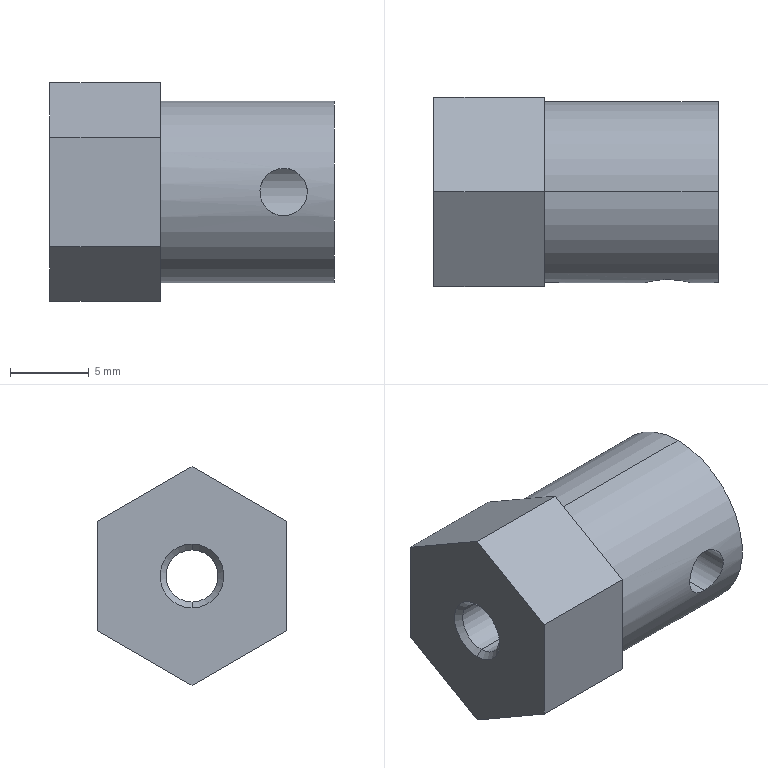Part | SolidWorks | features ICE 3, Extrusion 1, HoleWzd 1 | 1 solid | 20 faces | box 18 x 12 x 13.856 mm | volume 1793 mm3 | plane 10 | cylinder 8 | cone 2 | commonest cylinder face diameters 3 x2 3.3 x2 4 x2 11.5 x2
STEP:
#1=CARTESIAN_POINT('',(14.8,-5.551,-1.5));
#2=VERTEX_POINT('',#1);
#3=CARTESIAN_POINT('',(14.8,-5.551,1.5));
#4=VERTEX_POINT('',#3);
#5=CARTESIAN_POINT('',(14.8,-5.551,-1.5));
#6=CARTESIAN_POINT('',(14.604,-5.551,-1.5));
#7=CARTESIAN_POINT('',(14.406,-5.562,-1.46));
#8=CARTESIAN_POINT('',(14.135,-5.59,-1.348));
#9=CARTESIAN_POINT('',(14.047,-5.601,-1.301));
#10=CARTESIAN_POINT('',(13.884,-5.625,-1.192));
#11=CARTESIAN_POINT('',(13.809,-5.638,-1.13));
#12=CARTESIAN_POINT('',(13.671,-5.664,-0.992));
#13=CARTESIAN_POINT('',(13.608,-5.677,-0.9153));
#14=CARTESIAN_POINT('',(13.499,-5.701,-0.7534));
#15=CARTESIAN_POINT('',(13.453,-5.712,-0.6674));
#16=CARTESIAN_POINT('',(13.339,-5.739,-0.3935));
#17=CARTESIAN_POINT('',(13.3,-5.75,-0.1982));
#18=CARTESIAN_POINT('',(13.3,-5.75,0.09853));
#19=CARTESIAN_POINT('',(13.31,-5.747,0.1962));
#20=CARTESIAN_POINT('',(13.348,-5.738,0.389));
#21=CARTESIAN_POINT('',(13.377,-5.73,0.4847));
#22=CARTESIAN_POINT('',(13.49,-5.703,0.756));
#23=CARTESIAN_POINT('',(13.601,-5.677,0.9225));
#24=CARTESIAN_POINT('',(13.876,-5.626,1.198));
#25=CARTESIAN_POINT('',(14.043,-5.599,1.31));
#26=CARTESIAN_POINT('',(14.314,-5.571,1.422));
#27=CARTESIAN_POINT('',(14.409,-5.564,1.452));
#28=CARTESIAN_POINT('',(14.602,-5.554,1.49));
#29=CARTESIAN_POINT('',(14.7,-5.551,1.5));
#30=CARTESIAN_POINT('',(14.8,-5.551,1.5));
#31=B_SPLINE_CURVE_WITH_KNOTS('',3,(#5,#6,#7,#8,#9,#10,#11,#12,#13,#14,#15,#16,#17,#18,#19,#20,#21,#22,#23,#24,#25,#26,#27,#28,#29,#30),.UNSPECIFIED.,.F.,.F.,(4,2,2,2,2,2,2,2,2,2,2,2,4),(0.00471,0.005299,0.005593,0.005887,0.006182,0.006476,0.007064,0.007359,0.007653,0.008242,0.00883,0.009125,0.009419),.UNSPECIFIED.);
#32=EDGE_CURVE('',#2,#4,#31,.T.);
#33=ORIENTED_EDGE('',*,*,#32,.F.);
#34=CARTESIAN_POINT('',(14.8,-1.323,-1.5));
#35=VERTEX_POINT('',#34);
#36=CARTESIAN_POINT('',(14.8,-6.,-1.5));
#37=DIRECTION('',(0.,1.,0.));
#38=VECTOR('',#37,1000.);
#39=LINE('',#36,#38);
#40=EDGE_CURVE('',#2,#35,#39,.T.);
#41=ORIENTED_EDGE('',*,*,#40,.T.);
#42=CARTESIAN_POINT('',(14.8,-1.323,1.5));
#43=VERTEX_POINT('',#42);
#44=CARTESIAN_POINT('',(14.8,-1.323,1.5));
#45=CARTESIAN_POINT('',(14.696,-1.323,1.5));
#46=CARTESIAN_POINT('',(14.595,-1.335,1.489));
#47=CARTESIAN_POINT('',(14.399,-1.379,1.449));
#48=CARTESIAN_POINT('',(14.303,-1.411,1.419));
#49=CARTESIAN_POINT('',(14.037,-1.518,1.306));
#50=CARTESIAN_POINT('',(13.88,-1.608,1.2));
#51=CARTESIAN_POINT('',(13.679,-1.733,1.002));
#52=CARTESIAN_POINT('',(13.618,-1.774,0.9281));
#53=CARTESIAN_POINT('',(13.51,-1.847,0.7712));
#54=CARTESIAN_POINT('',(13.463,-1.881,0.6872));
#55=CARTESIAN_POINT('',(13.345,-1.966,0.4152));
#56=CARTESIAN_POINT('',(13.3,-2.,0.209));
#57=CARTESIAN_POINT('',(13.3,-2.,-0.2028));
#58=CARTESIAN_POINT('',(13.343,-1.967,-0.4078));
#59=CARTESIAN_POINT('',(13.499,-1.855,-0.7725));
#60=CARTESIAN_POINT('',(13.61,-1.776,-0.9331));
#61=CARTESIAN_POINT('',(13.812,-1.65,-1.133));
#62=CARTESIAN_POINT('',(13.884,-1.608,-1.192));
#63=CARTESIAN_POINT('',(14.04,-1.524,-1.297));
#64=CARTESIAN_POINT('',(14.124,-1.483,-1.343));
#65=CARTESIAN_POINT('',(14.391,-1.375,-1.456));
#66=CARTESIAN_POINT('',(14.592,-1.323,-1.5));
#67=CARTESIAN_POINT('',(14.8,-1.323,-1.5));
#68=B_SPLINE_CURVE_WITH_KNOTS('',3,(#44,#45,#46,#47,#48,#49,#50,#51,#52,#53,#54,#55,#56,#57,#58,#59,#60,#61,#62,#63,#64,#65,#66,#67),.UNSPECIFIED.,.F.,.F.,(4,2,2,2,2,2,2,2,2,2,2,4),(0.,0.0003062,0.0006124,0.001225,0.001531,0.001837,0.00245,0.003062,0.003675,0.003981,0.004287,0.004899),.UNSPECIFIED.);
#69=EDGE_CURVE('',#43,#35,#68,.T.);
#70=ORIENTED_EDGE('',*,*,#69,.F.);
#71=CARTESIAN_POINT('',(14.8,-6.,1.5));
#72=DIRECTION('',(0.,1.,0.));
#73=VECTOR('',#72,1000.);
#74=LINE('',#71,#73);
#75=EDGE_CURVE('',#4,#43,#74,.T.);
#76=ORIENTED_EDGE('',*,*,#75,.F.);
#77=EDGE_LOOP('',(#33,#41,#70,#76));
#78=FACE_OUTER_BOUND('',#77,.T.);
#79=CARTESIAN_POINT('',(14.8,-6.,0.));
#80=DIRECTION('',(0.,1.,0.));
#81=DIRECTION('',(0.,0.,1.));
#82=AXIS2_PLACEMENT_3D('',#79,#80,#81);
#83=CYLINDRICAL_SURFACE('',#82,1.5);
#84=ADVANCED_FACE('',(#78),#83,.F.);
#85=CARTESIAN_POINT('',(0.375,0.,-1.65));
#86=VERTEX_POINT('',#85);
#87=CARTESIAN_POINT('',(0.375,0.,1.65));
#88=VERTEX_POINT('',#87);
#89=CARTESIAN_POINT('',(0.375,0.,0.));
#90=DIRECTION('',(-1.,0.,0.));
#91=DIRECTION('',(0.,0.,1.));
#92=AXIS2_PLACEMENT_3D('',#89,#90,#91);
#93=CIRCLE('',#92,1.65);
#94=EDGE_CURVE('',#86,#88,#93,.T.);
#95=ORIENTED_EDGE('',*,*,#94,.F.);
#96=CARTESIAN_POINT('',(0.,0.,-2.025));
#97=VERTEX_POINT('',#96);
#98=CARTESIAN_POINT('',(0.,0.,-2.025));
#99=DIRECTION('',(-0.7071,0.,-0.7071));
#100=VECTOR('',#99,1000.);
#101=LINE('',#98,#100);
#102=EDGE_CURVE('',#86,#97,#101,.T.);
#103=ORIENTED_EDGE('',*,*,#102,.T.);
#104=CARTESIAN_POINT('',(0.,0.,2.025));
#105=VERTEX_POINT('',#104);
#106=CARTESIAN_POINT('',(0.,0.,0.));
#107=DIRECTION('',(-1.,0.,0.));
#108=DIRECTION('',(0.,0.,1.));
#109=AXIS2_PLACEMENT_3D('',#106,#107,#108);
#110=CIRCLE('',#109,2.025);
#111=EDGE_CURVE('',#97,#105,#110,.T.);
#112=ORIENTED_EDGE('',*,*,#111,.T.);
#113=CARTESIAN_POINT('',(0.,0.,2.025));
#114=DIRECTION('',(-0.7071,0.,0.7071));
#115=VECTOR('',#114,1000.);
#116=LINE('',#113,#115);
#117=EDGE_CURVE('',#88,#105,#116,.T.);
#118=ORIENTED_EDGE('',*,*,#117,.F.);
#119=EDGE_LOOP('',(#95,#103,#112,#118));
#120=FACE_OUTER_BOUND('',#119,.T.);
#121=CARTESIAN_POINT('',(0.,0.,0.));
#122=DIRECTION('',(-1.,0.,0.));
#123=DIRECTION('',(0.,0.,1.));
#124=AXIS2_PLACEMENT_3D('',#121,#122,#123);
#125=CONICAL_SURFACE('',#124,2.025,0.7854);
#126=ADVANCED_FACE('',(#120),#125,.F.);
#127=CARTESIAN_POINT('',(8.,0.,1.65));
#128=VERTEX_POINT('',#127);
#129=CARTESIAN_POINT('',(8.,0.,-1.65));
#130=VERTEX_POINT('',#129);
#131=CARTESIAN_POINT('',(8.,0.,0.));
#132=DIRECTION('',(1.,0.,0.));
#133=DIRECTION('',(0.,0.,-1.));
#134=AXIS2_PLACEMENT_3D('',#131,#132,#133);
#135=CIRCLE('',#134,1.65);
#136=EDGE_CURVE('',#128,#130,#135,.T.);
#137=ORIENTED_EDGE('',*,*,#136,.T.);
#138=CARTESIAN_POINT('',(0.,0.,-1.65));
#139=DIRECTION('',(-1.,0.,0.));
#140=VECTOR('',#139,1000.);
#141=LINE('',#138,#140);
#142=EDGE_CURVE('',#130,#86,#141,.T.);
#143=ORIENTED_EDGE('',*,*,#142,.T.);
#144=ORIENTED_EDGE('',*,*,#94,.T.);
#145=CARTESIAN_POINT('',(0.,0.,1.65));
#146=DIRECTION('',(-1.,0.,0.));
#147=VECTOR('',#146,1000.);
#148=LINE('',#145,#147);
#149=EDGE_CURVE('',#128,#88,#148,.T.);
#150=ORIENTED_EDGE('',*,*,#149,.F.);
#151=EDGE_LOOP('',(#137,#143,#144,#150));
#152=FACE_OUTER_BOUND('',#151,.T.);
#153=CARTESIAN_POINT('',(0.,0.,0.));
#154=DIRECTION('',(-1.,0.,0.));
#155=DIRECTION('',(0.,0.,1.));
#156=AXIS2_PLACEMENT_3D('',#153,#154,#155);
#157=CYLINDRICAL_SURFACE('',#156,1.65);
#158=ADVANCED_FACE('',(#152),#157,.F.);
#159=ORIENTED_EDGE('',*,*,#69,.T.);
#160=CARTESIAN_POINT('',(14.8,-1.323,-1.5));
#161=CARTESIAN_POINT('',(15.007,-1.323,-1.5));
#162=CARTESIAN_POINT('',(15.21,-1.375,-1.456));
#163=CARTESIAN_POINT('',(15.563,-1.519,-1.306));
#164=CARTESIAN_POINT('',(15.72,-1.608,-1.199));
#165=CARTESIAN_POINT('',(15.921,-1.733,-1.001));
#166=CARTESIAN_POINT('',(15.983,-1.774,-0.9276));
#167=CARTESIAN_POINT('',(16.09,-1.848,-0.7707));
#168=CARTESIAN_POINT('',(16.137,-1.881,-0.6867));
#169=CARTESIAN_POINT('',(16.255,-1.966,-0.4153));
#170=CARTESIAN_POINT('',(16.3,-2.,-0.2091));
#171=CARTESIAN_POINT('',(16.3,-2.,0.2031));
#172=CARTESIAN_POINT('',(16.257,-1.967,0.4079));
#173=CARTESIAN_POINT('',(16.101,-1.855,0.7722));
#174=CARTESIAN_POINT('',(15.99,-1.776,0.9327));
#175=CARTESIAN_POINT('',(15.788,-1.65,1.132));
#176=CARTESIAN_POINT('',(15.716,-1.608,1.192));
#177=CARTESIAN_POINT('',(15.56,-1.524,1.296));
#178=CARTESIAN_POINT('',(15.476,-1.483,1.342));
#179=CARTESIAN_POINT('',(15.21,-1.375,1.456));
#180=CARTESIAN_POINT('',(15.008,-1.323,1.5));
#181=CARTESIAN_POINT('',(14.8,-1.323,1.5));
#182=B_SPLINE_CURVE_WITH_KNOTS('',3,(#160,#161,#162,#163,#164,#165,#166,#167,#168,#169,#170,#171,#172,#173,#174,#175,#176,#177,#178,#179,#180,#181),.UNSPECIFIED.,.F.,.F.,(4,2,2,2,2,2,2,2,2,2,4),(0.004899,0.005511,0.006122,0.006427,0.006733,0.007344,0.007956,0.008567,0.008872,0.009178,0.009789),.UNSPECIFIED.);
#183=EDGE_CURVE('',#35,#43,#182,.T.);
#184=ORIENTED_EDGE('',*,*,#183,.T.);
#185=EDGE_LOOP('',(#159,#184));
#186=FACE_BOUND('',#185,.T.);
#187=CARTESIAN_POINT('',(8.,0.,2.));
#188=VERTEX_POINT('',#187);
#189=CARTESIAN_POINT('',(8.,0.,-2.));
#190=VERTEX_POINT('',#189);
#191=CARTESIAN_POINT('',(8.,0.,0.));
#192=DIRECTION('',(1.,0.,0.));
#193=DIRECTION('',(0.,0.,-1.));
#194=AXIS2_PLACEMENT_3D('',#191,#192,#193);
#195=CIRCLE('',#194,2.);
#196=EDGE_CURVE('',#188,#190,#195,.T.);
#197=ORIENTED_EDGE('',*,*,#196,.F.);
#198=CARTESIAN_POINT('',(18.,0.,2.));
#199=VERTEX_POINT('',#198);
#200=CARTESIAN_POINT('',(8.,0.,2.));
#201=DIRECTION('',(1.,0.,0.));
#202=VECTOR('',#201,1000.);
#203=LINE('',#200,#202);
#204=EDGE_CURVE('',#188,#199,#203,.T.);
#205=ORIENTED_EDGE('',*,*,#204,.T.);
#206=CARTESIAN_POINT('',(18.,0.,-2.));
#207=VERTEX_POINT('',#206);
#208=CARTESIAN_POINT('',(18.,0.,0.));
#209=DIRECTION('',(1.,0.,0.));
#210=DIRECTION('',(0.,0.,-1.));
#211=AXIS2_PLACEMENT_3D('',#208,#209,#210);
#212=CIRCLE('',#211,2.);
#213=EDGE_CURVE('',#199,#207,#212,.T.);
#214=ORIENTED_EDGE('',*,*,#213,.T.);
#215=CARTESIAN_POINT('',(8.,0.,-2.));
#216=DIRECTION('',(1.,0.,0.));
#217=VECTOR('',#216,1000.);
#218=LINE('',#215,#217);
#219=EDGE_CURVE('',#190,#207,#218,.T.);
#220=ORIENTED_EDGE('',*,*,#219,.F.);
#221=EDGE_LOOP('',(#197,#205,#214,#220));
#222=FACE_OUTER_BOUND('',#221,.T.);
#223=CARTESIAN_POINT('',(8.,0.,0.));
#224=DIRECTION('',(1.,0.,0.));
#225=DIRECTION('',(0.,0.,-1.));
#226=AXIS2_PLACEMENT_3D('',#223,#224,#225);
#227=CYLINDRICAL_SURFACE('',#226,2.);
#228=ADVANCED_FACE('',(#186,#222),#227,.F.);
#229=CARTESIAN_POINT('',(18.,0.,-5.75));
#230=VERTEX_POINT('',#229);
#231=CARTESIAN_POINT('',(18.,0.,5.75));
#232=VERTEX_POINT('',#231);
#233=CARTESIAN_POINT('',(18.,0.,0.));
#234=DIRECTION('',(1.,0.,0.));
#235=DIRECTION('',(0.,0.,-1.));
#236=AXIS2_PLACEMENT_3D('',#233,#234,#235);
#237=CIRCLE('',#236,5.75);
#238=EDGE_CURVE('',#230,#232,#237,.T.);
#239=ORIENTED_EDGE('',*,*,#238,.F.);
#240=CARTESIAN_POINT('',(7.,0.,-5.75));
#241=VERTEX_POINT('',#240);
#242=CARTESIAN_POINT('',(18.,0.,-5.75));
#243=DIRECTION('',(-1.,0.,0.));
#244=VECTOR('',#243,1000.);
#245=LINE('',#242,#244);
#246=EDGE_CURVE('',#230,#241,#245,.T.);
#247=ORIENTED_EDGE('',*,*,#246,.T.);
#248=CARTESIAN_POINT('',(7.,0.,5.75));
#249=VERTEX_POINT('',#248);
#250=CARTESIAN_POINT('',(7.,0.,0.));
#251=DIRECTION('',(1.,0.,0.));
#252=DIRECTION('',(0.,0.,-1.));
#253=AXIS2_PLACEMENT_3D('',#250,#251,#252);
#254=CIRCLE('',#253,5.75);
#255=EDGE_CURVE('',#241,#249,#254,.T.);
#256=ORIENTED_EDGE('',*,*,#255,.T.);
#257=CARTESIAN_POINT('',(18.,0.,5.75));
#258=DIRECTION('',(-1.,0.,0.));
#259=VECTOR('',#258,1000.);
#260=LINE('',#257,#259);
#261=EDGE_CURVE('',#232,#249,#260,.T.);
#262=ORIENTED_EDGE('',*,*,#261,.F.);
#263=EDGE_LOOP('',(#239,#247,#256,#262));
#264=FACE_OUTER_BOUND('',#263,.T.);
#265=CARTESIAN_POINT('',(18.,0.,0.));
#266=DIRECTION('',(-1.,0.,0.));
#267=DIRECTION('',(0.,0.,1.));
#268=AXIS2_PLACEMENT_3D('',#265,#266,#267);
#269=CYLINDRICAL_SURFACE('',#268,5.75);
#270=ADVANCED_FACE('',(#264),#269,.T.);
#271=CARTESIAN_POINT('',(0.,-6.,-3.464));
#272=VERTEX_POINT('',#271);
#273=CARTESIAN_POINT('',(0.,0.,-6.928));
#274=VERTEX_POINT('',#273);
#275=CARTESIAN_POINT('',(0.,-6.,-3.464));
#276=DIRECTION('',(0.,0.866,-0.5));
#277=VECTOR('',#276,1000.);
#278=LINE('',#275,#277);
#279=EDGE_CURVE('',#272,#274,#278,.T.);
#280=ORIENTED_EDGE('',*,*,#279,.F.);
#281=CARTESIAN_POINT('',(0.,-6.,3.464));
#282=VERTEX_POINT('',#281);
#283=CARTESIAN_POINT('',(0.,-6.,3.464));
#284=DIRECTION('',(0.,0.,-1.));
#285=VECTOR('',#284,1000.);
#286=LINE('',#283,#285);
#287=EDGE_CURVE('',#282,#272,#286,.T.);
#288=ORIENTED_EDGE('',*,*,#287,.F.);
#289=CARTESIAN_POINT('',(0.,0.,6.928));
#290=VERTEX_POINT('',#289);
#291=CARTESIAN_POINT('',(0.,0.,6.928));
#292=DIRECTION('',(0.,-0.866,-0.5));
#293=VECTOR('',#292,1000.);
#294=LINE('',#291,#293);
#295=EDGE_CURVE('',#290,#282,#294,.T.);
#296=ORIENTED_EDGE('',*,*,#295,.F.);
#297=CARTESIAN_POINT('',(0.,6.,3.464));
#298=VERTEX_POINT('',#297);
#299=CARTESIAN_POINT('',(0.,6.,3.464));
#300=DIRECTION('',(0.,-0.866,0.5));
#301=VECTOR('',#300,1000.);
#302=LINE('',#299,#301);
#303=EDGE_CURVE('',#298,#290,#302,.T.);
#304=ORIENTED_EDGE('',*,*,#303,.F.);
#305=CARTESIAN_POINT('',(0.,6.,-3.464));
#306=VERTEX_POINT('',#305);
#307=CARTESIAN_POINT('',(0.,6.,-3.464));
#308=DIRECTION('',(0.,0.,1.));
#309=VECTOR('',#308,1000.);
#310=LINE('',#307,#309);
#311=EDGE_CURVE('',#306,#298,#310,.T.);
#312=ORIENTED_EDGE('',*,*,#311,.F.);
#313=CARTESIAN_POINT('',(0.,0.,-6.928));
#314=DIRECTION('',(0.,0.866,0.5));
#315=VECTOR('',#314,1000.);
#316=LINE('',#313,#315);
#317=EDGE_CURVE('',#274,#306,#316,.T.);
#318=ORIENTED_EDGE('',*,*,#317,.F.);
#319=EDGE_LOOP('',(#280,#288,#296,#304,#312,#318));
#320=FACE_OUTER_BOUND('',#319,.T.);
#321=CARTESIAN_POINT('',(0.,0.,0.));
#322=DIRECTION('',(-1.,0.,0.));
#323=DIRECTION('',(0.,0.,1.));
#324=AXIS2_PLACEMENT_3D('',#321,#322,#323);
#325=CIRCLE('',#324,2.025);
#326=EDGE_CURVE('',#105,#97,#325,.T.);
#327=ORIENTED_EDGE('',*,*,#326,.F.);
#328=ORIENTED_EDGE('',*,*,#111,.F.);
#329=EDGE_LOOP('',(#327,#328));
#330=FACE_BOUND('',#329,.T.);
#331=CARTESIAN_POINT('',(0.,0.,0.));
#332=DIRECTION('',(1.,0.,0.));
#333=DIRECTION('',(0.,0.,-1.));
#334=AXIS2_PLACEMENT_3D('',#331,#332,#333);
#335=PLANE('',#334);
#336=ADVANCED_FACE('',(#320,#330),#335,.F.);
#337=ORIENTED_EDGE('',*,*,#279,.T.);
#338=CARTESIAN_POINT('',(7.,0.,-6.928));
#339=VERTEX_POINT('',#338);
#340=CARTESIAN_POINT('',(7.,0.,-6.928));
#341=DIRECTION('',(-1.,0.,0.));
#342=VECTOR('',#341,1000.);
#343=LINE('',#340,#342);
#344=EDGE_CURVE('',#339,#274,#343,.T.);
#345=ORIENTED_EDGE('',*,*,#344,.F.);
#346=CARTESIAN_POINT('',(7.,-6.,-3.464));
#347=VERTEX_POINT('',#346);
#348=CARTESIAN_POINT('',(7.,-6.,-3.464));
#349=DIRECTION('',(0.,0.866,-0.5));
#350=VECTOR('',#349,1000.);
#351=LINE('',#348,#350);
#352=EDGE_CURVE('',#347,#339,#351,.T.);
#353=ORIENTED_EDGE('',*,*,#352,.F.);
#354=CARTESIAN_POINT('',(7.,-6.,-3.464));
#355=DIRECTION('',(-1.,0.,0.));
#356=VECTOR('',#355,1000.);
#357=LINE('',#354,#356);
#358=EDGE_CURVE('',#347,#272,#357,.T.);
#359=ORIENTED_EDGE('',*,*,#358,.T.);
#360=EDGE_LOOP('',(#337,#345,#353,#359));
#361=FACE_OUTER_BOUND('',#360,.T.);
#362=CARTESIAN_POINT('',(7.,-6.,-3.464));
#363=DIRECTION('',(0.,0.5,0.866));
#364=DIRECTION('',(0.,-0.866,0.5));
#365=AXIS2_PLACEMENT_3D('',#362,#363,#364);
#366=PLANE('',#365);
#367=ADVANCED_FACE('',(#361),#366,.F.);
#368=ORIENTED_EDGE('',*,*,#317,.T.);
#369=CARTESIAN_POINT('',(7.,6.,-3.464));
#370=VERTEX_POINT('',#369);
#371=CARTESIAN_POINT('',(7.,6.,-3.464));
#372=DIRECTION('',(-1.,0.,0.));
#373=VECTOR('',#372,1000.);
#374=LINE('',#371,#373);
#375=EDGE_CURVE('',#370,#306,#374,.T.);
#376=ORIENTED_EDGE('',*,*,#375,.F.);
#377=CARTESIAN_POINT('',(7.,0.,-6.928));
#378=DIRECTION('',(0.,0.866,0.5));
#379=VECTOR('',#378,1000.);
#380=LINE('',#377,#379);
#381=EDGE_CURVE('',#339,#370,#380,.T.);
#382=ORIENTED_EDGE('',*,*,#381,.F.);
#383=ORIENTED_EDGE('',*,*,#344,.T.);
#384=EDGE_LOOP('',(#368,#376,#382,#383));
#385=FACE_OUTER_BOUND('',#384,.T.);
#386=CARTESIAN_POINT('',(7.,0.,-6.928));
#387=DIRECTION('',(0.,-0.5,0.866));
#388=DIRECTION('',(0.,-0.866,-0.5));
#389=AXIS2_PLACEMENT_3D('',#386,#387,#388);
#390=PLANE('',#389);
#391=ADVANCED_FACE('',(#385),#390,.F.);
#392=ORIENTED_EDGE('',*,*,#311,.T.);
#393=CARTESIAN_POINT('',(7.,6.,3.464));
#394=VERTEX_POINT('',#393);
#395=CARTESIAN_POINT('',(7.,6.,3.464));
#396=DIRECTION('',(-1.,0.,0.));
#397=VECTOR('',#396,1000.);
#398=LINE('',#395,#397);
#399=EDGE_CURVE('',#394,#298,#398,.T.);
#400=ORIENTED_EDGE('',*,*,#399,.F.);
#401=CARTESIAN_POINT('',(7.,6.,-3.464));
#402=DIRECTION('',(0.,0.,1.));
#403=VECTOR('',#402,1000.);
#404=LINE('',#401,#403);
#405=EDGE_CURVE('',#370,#394,#404,.T.);
#406=ORIENTED_EDGE('',*,*,#405,.F.);
#407=ORIENTED_EDGE('',*,*,#375,.T.);
#408=EDGE_LOOP('',(#392,#400,#406,#407));
#409=FACE_OUTER_BOUND('',#408,.T.);
#410=CARTESIAN_POINT('',(7.,6.,-3.464));
#411=DIRECTION('',(0.,-1.,0.));
#412=DIRECTION('',(0.,0.,-1.));
#413=AXIS2_PLACEMENT_3D('',#410,#411,#412);
#414=PLANE('',#413);
#415=ADVANCED_FACE('',(#409),#414,.F.);
#416=ORIENTED_EDGE('',*,*,#303,.T.);
#417=CARTESIAN_POINT('',(7.,0.,6.928));
#418=VERTEX_POINT('',#417);
#419=CARTESIAN_POINT('',(7.,0.,6.928));
#420=DIRECTION('',(-1.,0.,0.));
#421=VECTOR('',#420,1000.);
#422=LINE('',#419,#421);
#423=EDGE_CURVE('',#418,#290,#422,.T.);
#424=ORIENTED_EDGE('',*,*,#423,.F.);
#425=CARTESIAN_POINT('',(7.,6.,3.464));
#426=DIRECTION('',(0.,-0.866,0.5));
#427=VECTOR('',#426,1000.);
#428=LINE('',#425,#427);
#429=EDGE_CURVE('',#394,#418,#428,.T.);
#430=ORIENTED_EDGE('',*,*,#429,.F.);
#431=ORIENTED_EDGE('',*,*,#399,.T.);
#432=EDGE_LOOP('',(#416,#424,#430,#431));
#433=FACE_OUTER_BOUND('',#432,.T.);
#434=CARTESIAN_POINT('',(7.,6.,3.464));
#435=DIRECTION('',(0.,-0.5,-0.866));
#436=DIRECTION('',(0.,0.866,-0.5));
#437=AXIS2_PLACEMENT_3D('',#434,#435,#436);
#438=PLANE('',#437);
#439=ADVANCED_FACE('',(#433),#438,.F.);
#440=ORIENTED_EDGE('',*,*,#295,.T.);
#441=CARTESIAN_POINT('',(7.,-6.,3.464));
#442=VERTEX_POINT('',#441);
#443=CARTESIAN_POINT('',(7.,-6.,3.464));
#444=DIRECTION('',(-1.,0.,0.));
#445=VECTOR('',#444,1000.);
#446=LINE('',#443,#445);
#447=EDGE_CURVE('',#442,#282,#446,.T.);
#448=ORIENTED_EDGE('',*,*,#447,.F.);
#449=CARTESIAN_POINT('',(7.,0.,6.928));
#450=DIRECTION('',(0.,-0.866,-0.5));
#451=VECTOR('',#450,1000.);
#452=LINE('',#449,#451);
#453=EDGE_CURVE('',#418,#442,#452,.T.);
#454=ORIENTED_EDGE('',*,*,#453,.F.);
#455=ORIENTED_EDGE('',*,*,#423,.T.);
#456=EDGE_LOOP('',(#440,#448,#454,#455));
#457=FACE_OUTER_BOUND('',#456,.T.);
#458=CARTESIAN_POINT('',(7.,0.,6.928));
#459=DIRECTION('',(0.,0.5,-0.866));
#460=DIRECTION('',(0.,0.866,0.5));
#461=AXIS2_PLACEMENT_3D('',#458,#459,#460);
#462=PLANE('',#461);
#463=ADVANCED_FACE('',(#457),#462,.F.);
#464=ORIENTED_EDGE('',*,*,#287,.T.);
#465=ORIENTED_EDGE('',*,*,#358,.F.);
#466=CARTESIAN_POINT('',(7.,-6.,3.464));
#467=DIRECTION('',(0.,0.,-1.));
#468=VECTOR('',#467,1000.);
#469=LINE('',#466,#468);
#470=EDGE_CURVE('',#442,#347,#469,.T.);
#471=ORIENTED_EDGE('',*,*,#470,.F.);
#472=ORIENTED_EDGE('',*,*,#447,.T.);
#473=EDGE_LOOP('',(#464,#465,#471,#472));
#474=FACE_OUTER_BOUND('',#473,.T.);
#475=CARTESIAN_POINT('',(7.,-6.,3.464));
#476=DIRECTION('',(0.,1.,0.));
#477=DIRECTION('',(0.,0.,1.));
#478=AXIS2_PLACEMENT_3D('',#475,#476,#477);
#479=PLANE('',#478);
#480=ADVANCED_FACE('',(#474),#479,.F.);
#481=CARTESIAN_POINT('',(7.,0.,0.));
#482=DIRECTION('',(1.,0.,0.));
#483=DIRECTION('',(0.,0.,-1.));
#484=AXIS2_PLACEMENT_3D('',#481,#482,#483);
#485=CIRCLE('',#484,5.75);
#486=EDGE_CURVE('',#249,#241,#485,.T.);
#487=ORIENTED_EDGE('',*,*,#486,.F.);
#488=ORIENTED_EDGE('',*,*,#255,.F.);
#489=EDGE_LOOP('',(#487,#488));
#490=FACE_BOUND('',#489,.T.);
#491=ORIENTED_EDGE('',*,*,#352,.T.);
#492=ORIENTED_EDGE('',*,*,#381,.T.);
#493=ORIENTED_EDGE('',*,*,#405,.T.);
#494=ORIENTED_EDGE('',*,*,#429,.T.);
#495=ORIENTED_EDGE('',*,*,#453,.T.);
#496=ORIENTED_EDGE('',*,*,#470,.T.);
#497=EDGE_LOOP('',(#491,#492,#493,#494,#495,#496));
#498=FACE_OUTER_BOUND('',#497,.T.);
#499=CARTESIAN_POINT('',(7.,0.,0.));
#500=DIRECTION('',(1.,0.,0.));
#501=DIRECTION('',(0.,0.,-1.));
#502=AXIS2_PLACEMENT_3D('',#499,#500,#501);
#503=PLANE('',#502);
#504=ADVANCED_FACE('',(#490,#498),#503,.T.);
#505=ORIENTED_EDGE('',*,*,#246,.F.);
#506=CARTESIAN_POINT('',(18.,0.,0.));
#507=DIRECTION('',(1.,0.,0.));
#508=DIRECTION('',(0.,0.,-1.));
#509=AXIS2_PLACEMENT_3D('',#506,#507,#508);
#510=CIRCLE('',#509,5.75);
#511=EDGE_CURVE('',#232,#230,#510,.T.);
#512=ORIENTED_EDGE('',*,*,#511,.F.);
#513=ORIENTED_EDGE('',*,*,#261,.T.);
#514=ORIENTED_EDGE('',*,*,#486,.T.);
#515=EDGE_LOOP('',(#505,#512,#513,#514));
#516=FACE_OUTER_BOUND('',#515,.T.);
#517=CARTESIAN_POINT('',(14.8,-5.551,1.5));
#518=CARTESIAN_POINT('',(14.9,-5.551,1.5));
#519=CARTESIAN_POINT('',(14.997,-5.554,1.49));
#520=CARTESIAN_POINT('',(15.19,-5.564,1.452));
#521=CARTESIAN_POINT('',(15.285,-5.571,1.423));
#522=CARTESIAN_POINT('',(15.467,-5.59,1.347));
#523=CARTESIAN_POINT('',(15.553,-5.601,1.301));
#524=CARTESIAN_POINT('',(15.715,-5.625,1.192));
#525=CARTESIAN_POINT('',(15.792,-5.638,1.129));
#526=CARTESIAN_POINT('',(15.999,-5.677,0.9227));
#527=CARTESIAN_POINT('',(16.11,-5.703,0.756));
#528=CARTESIAN_POINT('',(16.26,-5.739,0.3953));
#529=CARTESIAN_POINT('',(16.3,-5.75,0.1973));
#530=CARTESIAN_POINT('',(16.3,-5.75,-0.0977));
#531=CARTESIAN_POINT('',(16.29,-5.747,-0.1976));
#532=CARTESIAN_POINT('',(16.252,-5.738,-0.3903));
#533=CARTESIAN_POINT('',(16.223,-5.73,-0.4841));
#534=CARTESIAN_POINT('',(16.11,-5.703,-0.7573));
#535=CARTESIAN_POINT('',(15.999,-5.677,-0.9222));
#536=CARTESIAN_POINT('',(15.791,-5.638,-1.13));
#537=CARTESIAN_POINT('',(15.716,-5.625,-1.192));
#538=CARTESIAN_POINT('',(15.553,-5.601,-1.301));
#539=CARTESIAN_POINT('',(15.466,-5.59,-1.348));
#540=CARTESIAN_POINT('',(15.285,-5.571,-1.423));
#541=CARTESIAN_POINT('',(15.191,-5.564,-1.451));
#542=CARTESIAN_POINT('',(14.998,-5.554,-1.49));
#543=CARTESIAN_POINT('',(14.898,-5.551,-1.5));
#544=CARTESIAN_POINT('',(14.8,-5.551,-1.5));
#545=B_SPLINE_CURVE_WITH_KNOTS('',3,(#517,#518,#519,#520,#521,#522,#523,#524,#525,#526,#527,#528,#529,#530,#531,#532,#533,#534,#535,#536,#537,#538,#539,#540,#541,#542,#543,#544),.UNSPECIFIED.,.F.,.F.,(4,2,2,2,2,2,2,2,2,2,2,2,2,4),(0.,0.0002944,0.0005888,0.0008831,0.001178,0.001766,0.002355,0.002649,0.002944,0.003533,0.003827,0.004121,0.004416,0.00471),.UNSPECIFIED.);
#546=EDGE_CURVE('',#4,#2,#545,.T.);
#547=ORIENTED_EDGE('',*,*,#546,.T.);
#548=ORIENTED_EDGE('',*,*,#32,.T.);
#549=EDGE_LOOP('',(#547,#548));
#550=FACE_BOUND('',#549,.T.);
#551=CARTESIAN_POINT('',(18.,0.,0.));
#552=DIRECTION('',(-1.,0.,0.));
#553=DIRECTION('',(0.,0.,1.));
#554=AXIS2_PLACEMENT_3D('',#551,#552,#553);
#555=CYLINDRICAL_SURFACE('',#554,5.75);
#556=ADVANCED_FACE('',(#516,#550),#555,.T.);
#557=CARTESIAN_POINT('',(18.,0.,0.));
#558=DIRECTION('',(1.,0.,0.));
#559=DIRECTION('',(0.,0.,-1.));
#560=AXIS2_PLACEMENT_3D('',#557,#558,#559);
#561=CIRCLE('',#560,2.);
#562=EDGE_CURVE('',#207,#199,#561,.T.);
#563=ORIENTED_EDGE('',*,*,#562,.F.);
#564=ORIENTED_EDGE('',*,*,#213,.F.);
#565=EDGE_LOOP('',(#563,#564));
#566=FACE_BOUND('',#565,.T.);
#567=ORIENTED_EDGE('',*,*,#511,.T.);
#568=ORIENTED_EDGE('',*,*,#238,.T.);
#569=EDGE_LOOP('',(#567,#568));
#570=FACE_OUTER_BOUND('',#569,.T.);
#571=CARTESIAN_POINT('',(18.,0.,0.));
#572=DIRECTION('',(1.,0.,0.));
#573=DIRECTION('',(0.,0.,-1.));
#574=AXIS2_PLACEMENT_3D('',#571,#572,#573);
#575=PLANE('',#574);
#576=ADVANCED_FACE('',(#566,#570),#575,.T.);
#577=ORIENTED_EDGE('',*,*,#204,.F.);
#578=CARTESIAN_POINT('',(8.,0.,0.));
#579=DIRECTION('',(1.,0.,0.));
#580=DIRECTION('',(0.,0.,-1.));
#581=AXIS2_PLACEMENT_3D('',#578,#579,#580);
#582=CIRCLE('',#581,2.);
#583=EDGE_CURVE('',#190,#188,#582,.T.);
#584=ORIENTED_EDGE('',*,*,#583,.F.);
#585=ORIENTED_EDGE('',*,*,#219,.T.);
#586=ORIENTED_EDGE('',*,*,#562,.T.);
#587=EDGE_LOOP('',(#577,#584,#585,#586));
#588=FACE_OUTER_BOUND('',#587,.T.);
#589=CARTESIAN_POINT('',(8.,0.,0.));
#590=DIRECTION('',(1.,0.,0.));
#591=DIRECTION('',(0.,0.,-1.));
#592=AXIS2_PLACEMENT_3D('',#589,#590,#591);
#593=CYLINDRICAL_SURFACE('',#592,2.);
#594=ADVANCED_FACE('',(#588),#593,.F.);
#595=ORIENTED_EDGE('',*,*,#136,.F.);
#596=CARTESIAN_POINT('',(8.,0.,0.));
#597=DIRECTION('',(1.,0.,0.));
#598=DIRECTION('',(0.,0.,-1.));
#599=AXIS2_PLACEMENT_3D('',#596,#597,#598);
#600=CIRCLE('',#599,1.65);
#601=EDGE_CURVE('',#130,#128,#600,.T.);
#602=ORIENTED_EDGE('',*,*,#601,.F.);
#603=EDGE_LOOP('',(#595,#602));
#604=FACE_BOUND('',#603,.T.);
#605=ORIENTED_EDGE('',*,*,#583,.T.);
#606=ORIENTED_EDGE('',*,*,#196,.T.);
#607=EDGE_LOOP('',(#605,#606));
#608=FACE_OUTER_BOUND('',#607,.T.);
#609=CARTESIAN_POINT('',(8.,0.,0.));
#610=DIRECTION('',(1.,0.,0.));
#611=DIRECTION('',(0.,0.,-1.));
#612=AXIS2_PLACEMENT_3D('',#609,#610,#611);
#613=PLANE('',#612);
#614=ADVANCED_FACE('',(#604,#608),#613,.T.);
#615=ORIENTED_EDGE('',*,*,#142,.F.);
#616=ORIENTED_EDGE('',*,*,#601,.T.);
#617=ORIENTED_EDGE('',*,*,#149,.T.);
#618=CARTESIAN_POINT('',(0.375,0.,0.));
#619=DIRECTION('',(-1.,0.,0.));
#620=DIRECTION('',(0.,0.,1.));
#621=AXIS2_PLACEMENT_3D('',#618,#619,#620);
#622=CIRCLE('',#621,1.65);
#623=EDGE_CURVE('',#88,#86,#622,.T.);
#624=ORIENTED_EDGE('',*,*,#623,.T.);
#625=EDGE_LOOP('',(#615,#616,#617,#624));
#626=FACE_OUTER_BOUND('',#625,.T.);
#627=CARTESIAN_POINT('',(0.,0.,0.));
#628=DIRECTION('',(-1.,0.,0.));
#629=DIRECTION('',(0.,0.,1.));
#630=AXIS2_PLACEMENT_3D('',#627,#628,#629);
#631=CYLINDRICAL_SURFACE('',#630,1.65);
#632=ADVANCED_FACE('',(#626),#631,.F.);
#633=ORIENTED_EDGE('',*,*,#102,.F.);
#634=ORIENTED_EDGE('',*,*,#623,.F.);
#635=ORIENTED_EDGE('',*,*,#117,.T.);
#636=ORIENTED_EDGE('',*,*,#326,.T.);
#637=EDGE_LOOP('',(#633,#634,#635,#636));
#638=FACE_OUTER_BOUND('',#637,.T.);
#639=CARTESIAN_POINT('',(0.,0.,0.));
#640=DIRECTION('',(-1.,0.,0.));
#641=DIRECTION('',(0.,0.,1.));
#642=AXIS2_PLACEMENT_3D('',#639,#640,#641);
#643=CONICAL_SURFACE('',#642,2.025,0.7854);
#644=ADVANCED_FACE('',(#638),#643,.F.);
#645=ORIENTED_EDGE('',*,*,#40,.F.);
#646=ORIENTED_EDGE('',*,*,#546,.F.);
#647=ORIENTED_EDGE('',*,*,#75,.T.);
#648=ORIENTED_EDGE('',*,*,#183,.F.);
#649=EDGE_LOOP('',(#645,#646,#647,#648));
#650=FACE_OUTER_BOUND('',#649,.T.);
#651=CARTESIAN_POINT('',(14.8,-6.,0.));
#652=DIRECTION('',(0.,1.,0.));
#653=DIRECTION('',(0.,0.,1.));
#654=AXIS2_PLACEMENT_3D('',#651,#652,#653);
#655=CYLINDRICAL_SURFACE('',#654,1.5);
#656=ADVANCED_FACE('',(#650),#655,.F.);
#657=CLOSED_SHELL('',(#84,#126,#158,#228,#270,#336,#367,#391,#415,#439,#463,#480,#504,#556,#576,#594,#614,#632,#644,#656));
#658=MANIFOLD_SOLID_BREP('',#657);
#659=CARTESIAN_POINT('',(0.,0.,0.));
#660=DIRECTION('',(0.,0.,1.));
#661=DIRECTION('',(1.,0.,0.));
#662=AXIS2_PLACEMENT_3D('',#659,#660,#661);
#663=(LENGTH_UNIT()NAMED_UNIT(*)SI_UNIT(.MILLI.,.METRE.));
#664=UNCERTAINTY_MEASURE_WITH_UNIT(LENGTH_MEASURE(0.00001),#663,'','');
#665=(NAMED_UNIT(*)PLANE_ANGLE_UNIT()SI_UNIT($,.RADIAN.));
#666=(NAMED_UNIT(*)SI_UNIT($,.STERADIAN.)SOLID_ANGLE_UNIT());
#667=(GEOMETRIC_REPRESENTATION_CONTEXT(3)GLOBAL_UNCERTAINTY_ASSIGNED_CONTEXT((#664))GLOBAL_UNIT_ASSIGNED_CONTEXT((#663,#665,#666))REPRESENTATION_CONTEXT('',''));
#668=ADVANCED_BREP_SHAPE_REPRESENTATION('',(#658,#662),#667);